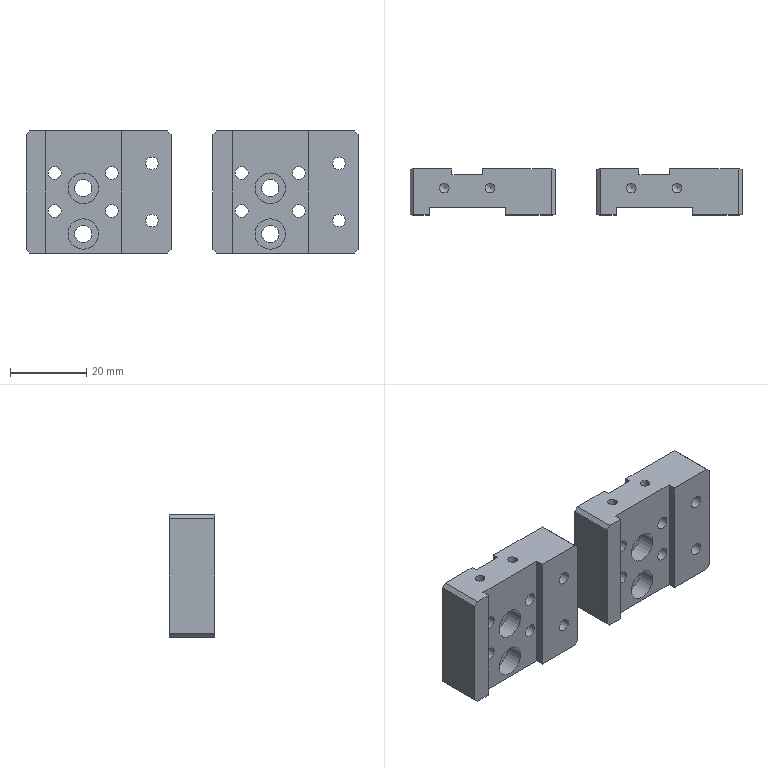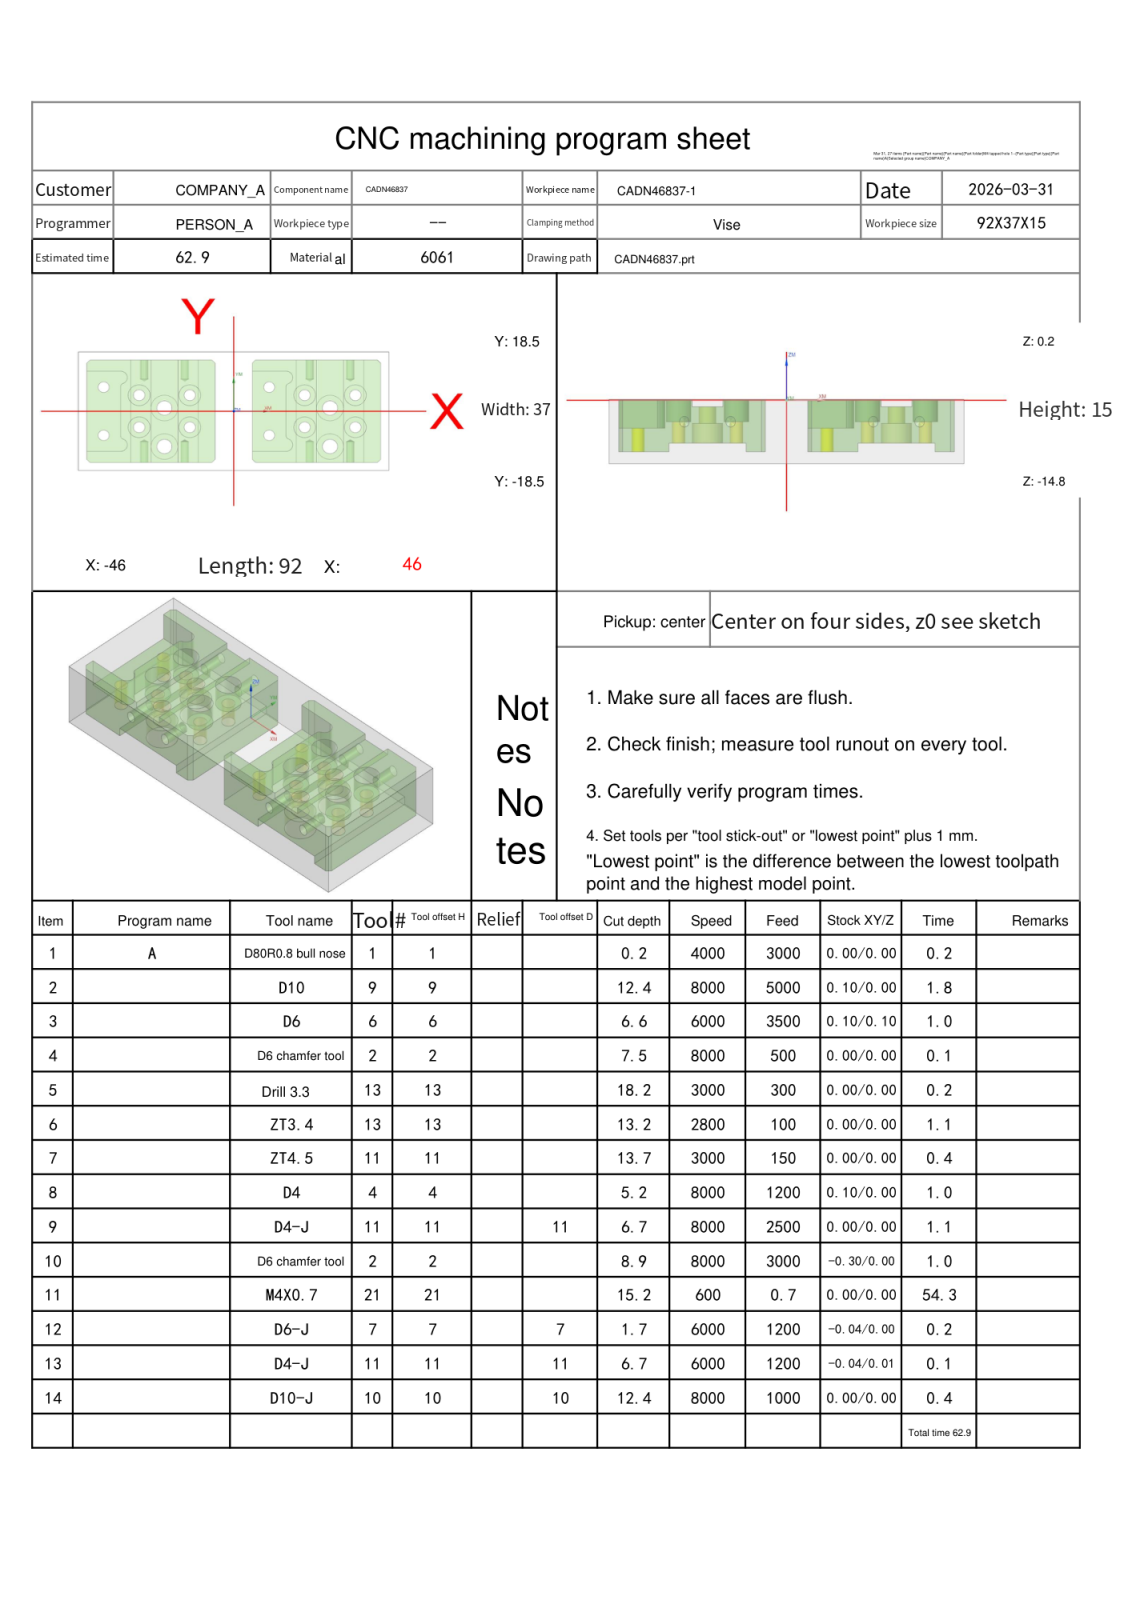NC program | NX | posted by the shop | part box 87 x 12 x 32 mm
Lines 2026 to 3069 of 5636:
N9 T11 M06
(D4-J  D=4. R=0. H=11 ce=0.00 di=0.00)
G00 G90 G54 X-28. Y5. M03 S8000
G43 H11 Z20.
M08
Z.5
G41 D11
G01 X-28.062 Y5.19 F500.
G03 X-28.641 Y5.609 I-.579 J-.19
X-29.25 Y5. I0.0 J-.609
X-29.25 Y5. Z-4.5 I1.25 J0.0
X-29.011 Y4.265 Z-5. I1.25 J0.0
X-28. Y3.75 I1.011 J.735
X-26.75 Y5. I0.0 J1.25
X-28. Y6.25 I-1.25 J0.0
X-29.25 Y5. I0.0 J-1.25
X-29.011 Y4.265 I1.25 J0.0
X-28.519 Y4.014 I.493 J.358
X-27.91 Y4.623 I0.0 J.609
G01 X-27.939 Y4.81
G40 X-28. Y5.
G00 Z20.
Y-5.
Z.5
G41 D11
G01 X-28.062 Y-4.81
G03 X-28.641 Y-4.391 I-.579 J-.19
X-29.25 Y-5. I0.0 J-.609
X-29.25 Y-5. Z-4.5 I1.25 J0.0
X-29.011 Y-5.735 Z-5. I1.25 J0.0
X-28. Y-6.25 I1.011 J.735
X-26.75 Y-5. I0.0 J1.25
X-28. Y-3.75 I-1.25 J0.0
X-29.25 Y-5. I0.0 J-1.25
X-29.011 Y-5.735 I1.25 J0.0
X-28.519 Y-5.986 I.493 J.358
X-27.91 Y-5.377 I0.0 J.609
G01 X-27.939 Y-5.19
G40 X-28. Y-5.
G00 Z20.
X-13.
Z.5
G41 D11
G01 X-13.062 Y-4.81
G03 X-13.641 Y-4.391 I-.579 J-.19
X-14.25 Y-5. I0.0 J-.609
X-14.25 Y-5. Z-4.5 I1.25 J0.0
X-14.011 Y-5.735 Z-5. I1.25 J0.0
X-13. Y-6.25 I1.011 J.735
X-11.75 Y-5. I0.0 J1.25
X-13. Y-3.75 I-1.25 J0.0
X-14.25 Y-5. I0.0 J-1.25
X-14.011 Y-5.735 I1.25 J0.0
X-13.519 Y-5.986 I.493 J.358
X-12.91 Y-5.377 I0.0 J.609
G01 X-12.939 Y-5.19
G40 X-13. Y-5.
G00 Z20.
Y5.
Z.5
G41 D11
G01 X-13.062 Y5.19
G03 X-13.641 Y5.609 I-.579 J-.19
X-14.25 Y5. I0.0 J-.609
X-14.25 Y5. Z-4.5 I1.25 J0.0
X-14.011 Y4.265 Z-5. I1.25 J0.0
X-13. Y3.75 I1.011 J.735
X-11.75 Y5. I0.0 J1.25
X-13. Y6.25 I-1.25 J0.0
X-14.25 Y5. I0.0 J-1.25
X-14.011 Y4.265 I1.25 J0.0
X-13.519 Y4.014 I.493 J.358
X-12.91 Y4.623 I0.0 J.609
G01 X-12.939 Y4.81
G40 X-13. Y5.
G00 Z20.
X21.
Z.5
G41 D11
G01 X20.938 Y5.19
G03 X20.359 Y5.609 I-.579 J-.19
X19.75 Y5. I0.0 J-.609
X19.75 Y5. Z-4.5 I1.25 J0.0
X19.989 Y4.265 Z-5. I1.25 J0.0
X21. Y3.75 I1.011 J.735
X22.25 Y5. I0.0 J1.25
X21. Y6.25 I-1.25 J0.0
X19.75 Y5. I0.0 J-1.25
X19.989 Y4.265 I1.25 J0.0
X20.481 Y4.014 I.493 J.358
X21.09 Y4.623 I0.0 J.609
G01 X21.061 Y4.81
G40 X21. Y5.
G00 Z20.
Y-5.
Z.5
G41 D11
G01 X20.938 Y-4.81
G03 X20.359 Y-4.391 I-.579 J-.19
X19.75 Y-5. I0.0 J-.609
X19.75 Y-5. Z-4.5 I1.25 J0.0
X19.989 Y-5.735 Z-5. I1.25 J0.0
X21. Y-6.25 I1.011 J.735
X22.25 Y-5. I0.0 J1.25
X21. Y-3.75 I-1.25 J0.0
X19.75 Y-5. I0.0 J-1.25
X19.989 Y-5.735 I1.25 J0.0
X20.481 Y-5.986 I.493 J.358
X21.09 Y-5.377 I0.0 J.609
G01 X21.061 Y-5.19
G40 X21. Y-5.
G00 Z20.
X36.
Z.5
G41 D11
G01 X35.938 Y-4.81
G03 X35.359 Y-4.391 I-.579 J-.19
X34.75 Y-5. I0.0 J-.609
X34.75 Y-5. Z-4.5 I1.25 J0.0
X34.989 Y-5.735 Z-5. I1.25 J0.0
X36. Y-6.25 I1.011 J.735
X37.25 Y-5. I0.0 J1.25
X36. Y-3.75 I-1.25 J0.0
X34.75 Y-5. I0.0 J-1.25
X34.989 Y-5.735 I1.25 J0.0
X35.481 Y-5.986 I.493 J.358
X36.09 Y-5.377 I0.0 J.609
G01 X36.061 Y-5.19
G40 X36. Y-5.
G00 Z20.
Y5.
Z.5
G41 D11
G01 X35.938 Y5.19
G03 X35.359 Y5.609 I-.579 J-.19
X34.75 Y5. I0.0 J-.609
X34.75 Y5. Z-4.5 I1.25 J0.0
X34.989 Y4.265 Z-5. I1.25 J0.0
X36. Y3.75 I1.011 J.735
X37.25 Y5. I0.0 J1.25
X36. Y6.25 I-1.25 J0.0
X34.75 Y5. I0.0 J-1.25
X34.989 Y4.265 I1.25 J0.0
X35.481 Y4.014 I.493 J.358
X36.09 Y4.623 I0.0 J.609
G01 X36.061 Y4.81
G40 X36. Y5.
G00 Z20.
G00 G90 X-39.064 Y-9.895 M03 S6000
Z20.
Z.305
G01 X-39.063 Y-9.902 Z.219 F2000.
X-39.059 Y-9.921 Z.141
X-39.053 Y-9.951 Z.071
X-39.045 Y-9.989 Z.009
X-39.033 Y-10.035 Z-.047
X-39.018 Y-10.086 Z-.096
X-39. Y-10.141 Z-.139
X-38.978 Y-10.197 Z-.175
X-38.953 Y-10.254 Z-.206
X-38.924 Y-10.309 Z-.232
X-38.89 Y-10.36 Z-.253
X-38.852 Y-10.405 Z-.269
X-38.81 Y-10.444 Z-.281
X-38.763 Y-10.474 Z-.289
X-38.71 Y-10.493 Z-.294
X-38.653 Y-10.5 Z-.295
X-33.5 F2500.
G02 X-35.5 Y-7.672 I1. J2.828
G01 Y-7.316
X-35.516 Y-7.273 Z-.296
X-35.562 Y-7.252 Z-.299
X-35.634 Y-7.251 Z-.303
X-35.73 Y-7.27 Z-.308
X-35.844 Y-7.305 Z-.315
X-35.975 Y-7.356 Z-.323
X-36.119 Y-7.42 Z-.332
X-36.272 Y-7.496 Z-.342
X-36.514 Y-7.632 Z-.358
X-36.753 Y-7.781 Z-.375
X-37.091 Y-8.025 Z-.402
X-37.407 Y-8.295 Z-.429
X-37.7 Y-8.588 Z-.457
X-37.967 Y-8.905 Z-.484
X-38.208 Y-9.244 Z-.51
X-38.309 Y-9.405 Z-.522
X-38.402 Y-9.566 Z-.533
X-38.486 Y-9.726 Z-.544
X-38.56 Y-9.879 Z-.554
X-38.622 Y-10.023 Z-.563
X-38.67 Y-10.155 Z-.57
X-38.704 Y-10.27 Z-.577
X-38.72 Y-10.365 Z-.583
X-38.718 Y-10.438 Z-.587
X-38.696 Y-10.484 Z-.59
X-38.653 Y-10.5
X-33.5
G02 X-35.5 Y-7.672 I1. J2.828
G01 Y-7.316
X-35.516 Y-7.273 Z-.591
X-35.562 Y-7.252 Z-.594
X-35.634 Y-7.251 Z-.598
X-35.73 Y-7.27 Z-.604
X-35.844 Y-7.305 Z-.61
X-35.975 Y-7.356 Z-.618
X-36.119 Y-7.42 Z-.627
X-36.272 Y-7.496 Z-.637
X-36.514 Y-7.632 Z-.653
X-36.753 Y-7.781 Z-.67
X-37.091 Y-8.025 Z-.697
X-37.407 Y-8.295 Z-.724
X-37.7 Y-8.588 Z-.752
X-37.967 Y-8.905 Z-.779
X-38.208 Y-9.244 Z-.806
X-38.309 Y-9.405 Z-.817
X-38.402 Y-9.566 Z-.828
X-38.486 Y-9.726 Z-.839
X-38.56 Y-9.879 Z-.849
X-38.622 Y-10.023 Z-.858
X-38.67 Y-10.155 Z-.866
X-38.704 Y-10.27 Z-.873
X-38.72 Y-10.365 Z-.878
X-38.718 Y-10.438 Z-.882
X-38.696 Y-10.484 Z-.885
X-38.653 Y-10.5 Z-.886
X-33.5
G02 X-35.5 Y-7.672 I1. J2.828
G01 Y-7.316
X-35.516 Y-7.273 Z-.887
X-35.562 Y-7.252 Z-.889
X-35.634 Y-7.251 Z-.893
X-35.73 Y-7.27 Z-.899
X-35.844 Y-7.305 Z-.906
X-35.975 Y-7.356 Z-.914
X-36.119 Y-7.42 Z-.923
X-36.272 Y-7.496 Z-.932
X-36.514 Y-7.632 Z-.949
X-36.753 Y-7.781 Z-.966
X-37.091 Y-8.025 Z-.992
X-37.407 Y-8.295 Z-1.019
X-37.7 Y-8.588 Z-1.047
X-37.967 Y-8.905 Z-1.074
X-38.208 Y-9.244 Z-1.101
X-38.309 Y-9.405 Z-1.113
X-38.402 Y-9.566 Z-1.124
X-38.486 Y-9.726 Z-1.134
X-38.56 Y-9.879 Z-1.144
X-38.622 Y-10.023 Z-1.153
X-38.67 Y-10.155 Z-1.161
X-38.704 Y-10.27 Z-1.168
X-38.72 Y-10.365 Z-1.173
X-38.718 Y-10.438 Z-1.177
X-38.696 Y-10.484 Z-1.18
X-38.653 Y-10.5 Z-1.181
X-33.5
G02 X-35.5 Y-7.672 I1. J2.828
G01 Y-7.316
X-35.516 Y-7.273 Z-1.182
X-35.562 Y-7.252 Z-1.184
X-35.634 Y-7.251 Z-1.189
X-35.73 Y-7.27 Z-1.194
X-35.844 Y-7.305 Z-1.201
X-35.975 Y-7.356 Z-1.209
X-36.119 Y-7.42 Z-1.218
X-36.272 Y-7.496 Z-1.228
X-36.514 Y-7.632 Z-1.244
X-36.753 Y-7.781 Z-1.261
X-37.091 Y-8.025 Z-1.287
X-37.407 Y-8.295 Z-1.315
X-37.7 Y-8.588 Z-1.342
X-37.967 Y-8.905 Z-1.37
X-38.208 Y-9.244 Z-1.396
X-38.309 Y-9.405 Z-1.408
X-38.402 Y-9.566 Z-1.419
X-38.486 Y-9.726 Z-1.429
X-38.56 Y-9.879 Z-1.439
X-38.622 Y-10.023 Z-1.448
X-38.67 Y-10.155 Z-1.456
X-38.704 Y-10.27 Z-1.463
X-38.72 Y-10.365 Z-1.469
X-38.718 Y-10.438 Z-1.473
X-38.696 Y-10.484 Z-1.475
X-38.653 Y-10.5 Z-1.476
X-33.5
G02 X-35.5 Y-7.672 I1. J2.828
G01 Y-7.316
X-35.516 Y-7.273 Z-1.477
X-35.562 Y-7.252 Z-1.48
X-35.634 Y-7.251 Z-1.484
X-35.73 Y-7.27 Z-1.489
X-35.844 Y-7.305 Z-1.496
X-35.975 Y-7.356 Z-1.504
X-36.119 Y-7.42 Z-1.513
X-36.272 Y-7.496 Z-1.523
X-36.514 Y-7.632 Z-1.539
X-36.753 Y-7.781 Z-1.556
X-37.091 Y-8.025 Z-1.583
X-37.407 Y-8.295 Z-1.61
X-37.7 Y-8.588 Z-1.638
X-37.967 Y-8.905 Z-1.665
X-38.208 Y-9.244 Z-1.691
X-38.309 Y-9.405 Z-1.703
X-38.402 Y-9.566 Z-1.714
X-38.486 Y-9.726 Z-1.725
X-38.56 Y-9.879 Z-1.734
X-38.622 Y-10.023 Z-1.743
X-38.67 Y-10.155 Z-1.751
X-38.704 Y-10.27 Z-1.758
X-38.72 Y-10.365 Z-1.764
X-38.718 Y-10.438 Z-1.768
X-38.696 Y-10.484 Z-1.77
X-38.653 Y-10.5 Z-1.771
X-33.5
G02 X-35.5 Y-7.672 I1. J2.828
G01 Y-7.316
X-35.516 Y-7.273 Z-1.772
X-35.562 Y-7.252 Z-1.775
X-35.634 Y-7.251 Z-1.779
X-35.73 Y-7.27 Z-1.785
X-35.844 Y-7.305 Z-1.791
X-35.975 Y-7.356 Z-1.799
X-36.119 Y-7.42 Z-1.808
X-36.272 Y-7.496 Z-1.818
X-36.514 Y-7.632 Z-1.834
X-36.753 Y-7.781 Z-1.851
X-37.091 Y-8.025 Z-1.878
X-37.407 Y-8.295 Z-1.905
X-37.7 Y-8.588 Z-1.933
X-37.967 Y-8.905 Z-1.96
X-38.208 Y-9.244 Z-1.987
X-38.309 Y-9.405 Z-1.998
X-38.402 Y-9.566 Z-2.009
X-38.486 Y-9.726 Z-2.02
X-38.56 Y-9.879 Z-2.03
X-38.622 Y-10.023 Z-2.039
X-38.67 Y-10.155 Z-2.047
X-38.704 Y-10.27 Z-2.053
X-38.72 Y-10.365 Z-2.059
X-38.718 Y-10.438 Z-2.063
X-38.696 Y-10.484 Z-2.066
X-38.653 Y-10.5 Z-2.067
X-33.5
G02 X-35.5 Y-7.672 I1. J2.828
G01 Y-7.316
X-35.516 Y-7.273
X-35.562 Y-7.252 Z-2.07
X-35.634 Y-7.251 Z-2.074
X-35.73 Y-7.27 Z-2.08
X-35.844 Y-7.305 Z-2.087
X-35.975 Y-7.356 Z-2.095
X-36.119 Y-7.42 Z-2.103
X-36.272 Y-7.496 Z-2.113
X-36.514 Y-7.632 Z-2.13
X-36.753 Y-7.781 Z-2.147
X-37.091 Y-8.025 Z-2.173
X-37.407 Y-8.295 Z-2.2
X-37.7 Y-8.588 Z-2.228
X-37.967 Y-8.905 Z-2.255
X-38.208 Y-9.244 Z-2.282
X-38.309 Y-9.405 Z-2.293
X-38.402 Y-9.566 Z-2.305
X-38.486 Y-9.726 Z-2.315
X-38.56 Y-9.879 Z-2.325
X-38.622 Y-10.023 Z-2.334
X-38.67 Y-10.155 Z-2.342
X-38.704 Y-10.27 Z-2.349
X-38.72 Y-10.365 Z-2.354
X-38.718 Y-10.438 Z-2.358
X-38.696 Y-10.484 Z-2.361
X-38.653 Y-10.5 Z-2.362
X-33.5
G02 X-35.5 Y-7.672 I1. J2.828
G01 Y-7.316
X-35.516 Y-7.273 Z-2.363
X-35.562 Y-7.252 Z-2.365
X-35.634 Y-7.251 Z-2.369
X-35.73 Y-7.27 Z-2.375
X-35.844 Y-7.305 Z-2.382
X-35.975 Y-7.356 Z-2.39
X-36.119 Y-7.42 Z-2.399
X-36.272 Y-7.496 Z-2.409
X-36.514 Y-7.632 Z-2.425
X-36.753 Y-7.781 Z-2.442
X-37.091 Y-8.025 Z-2.468
X-37.407 Y-8.295 Z-2.496
X-37.7 Y-8.588 Z-2.523
X-37.967 Y-8.905 Z-2.551
X-38.208 Y-9.244 Z-2.577
X-38.309 Y-9.405 Z-2.589
X-38.402 Y-9.566 Z-2.6
X-38.486 Y-9.726 Z-2.61
X-38.56 Y-9.879 Z-2.62
X-38.622 Y-10.023 Z-2.629
X-38.67 Y-10.155 Z-2.637
X-38.704 Y-10.27 Z-2.644
X-38.72 Y-10.365 Z-2.649
X-38.718 Y-10.438 Z-2.654
X-38.696 Y-10.484 Z-2.656
X-38.653 Y-10.5 Z-2.657
X-33.5
G02 X-35.5 Y-7.672 I1. J2.828
G01 Y-7.316
X-35.516 Y-7.273 Z-2.658
X-35.562 Y-7.252 Z-2.661
X-35.634 Y-7.251 Z-2.665
X-35.73 Y-7.27 Z-2.67
X-35.844 Y-7.305 Z-2.677
X-35.975 Y-7.356 Z-2.685
X-36.119 Y-7.42 Z-2.694
X-36.272 Y-7.496 Z-2.704
X-36.514 Y-7.632 Z-2.72
X-36.753 Y-7.781 Z-2.737
X-37.091 Y-8.025 Z-2.763
X-37.407 Y-8.295 Z-2.791
X-37.7 Y-8.588 Z-2.818
X-37.967 Y-8.905 Z-2.846
X-38.208 Y-9.244 Z-2.872
X-38.309 Y-9.405 Z-2.884
X-38.402 Y-9.566 Z-2.895
X-38.486 Y-9.726 Z-2.906
X-38.56 Y-9.879 Z-2.915
X-38.622 Y-10.023 Z-2.924
X-38.67 Y-10.155 Z-2.932
X-38.704 Y-10.27 Z-2.939
X-38.72 Y-10.365 Z-2.945
X-38.718 Y-10.438 Z-2.949
X-38.696 Y-10.484 Z-2.951
X-38.653 Y-10.5 Z-2.952
X-33.5
G02 X-35.5 Y-7.672 I1. J2.828
G01 Y-7.316
X-35.516 Y-7.273 Z-2.953
X-35.562 Y-7.252 Z-2.956
X-35.634 Y-7.251 Z-2.96
X-35.73 Y-7.27 Z-2.965
X-35.844 Y-7.305 Z-2.972
X-35.975 Y-7.356 Z-2.98
X-36.119 Y-7.42 Z-2.989
X-36.272 Y-7.496 Z-2.999
X-36.514 Y-7.632 Z-3.015
X-36.753 Y-7.781 Z-3.032
X-37.091 Y-8.025 Z-3.059
X-37.407 Y-8.295 Z-3.086
X-37.7 Y-8.588 Z-3.114
X-37.967 Y-8.905 Z-3.141
X-38.208 Y-9.244 Z-3.168
X-38.309 Y-9.405 Z-3.179
X-38.402 Y-9.566 Z-3.19
X-38.486 Y-9.726 Z-3.201
X-38.56 Y-9.879 Z-3.211
X-38.622 Y-10.023 Z-3.22
X-38.67 Y-10.155 Z-3.228
X-38.704 Y-10.27 Z-3.234
X-38.72 Y-10.365 Z-3.24
X-38.718 Y-10.438 Z-3.244
X-38.696 Y-10.484 Z-3.247
X-38.653 Y-10.5 Z-3.248
X-33.5
G02 X-35.5 Y-7.672 I1. J2.828
G01 Y-7.316
X-35.516 Y-7.273
X-35.562 Y-7.252 Z-3.251
X-35.634 Y-7.251 Z-3.255
X-35.73 Y-7.27 Z-3.261
X-35.844 Y-7.305 Z-3.267
X-35.975 Y-7.356 Z-3.275
X-36.119 Y-7.42 Z-3.284
X-36.272 Y-7.496 Z-3.294
X-36.514 Y-7.632 Z-3.31
X-36.753 Y-7.781 Z-3.327
X-37.091 Y-8.025 Z-3.354
X-37.407 Y-8.295 Z-3.381
X-37.7 Y-8.588 Z-3.409
X-37.967 Y-8.905 Z-3.436
X-38.208 Y-9.244 Z-3.463
X-38.309 Y-9.405 Z-3.474
X-38.402 Y-9.566 Z-3.485
X-38.486 Y-9.726 Z-3.496
X-38.56 Y-9.879 Z-3.506
X-38.622 Y-10.023 Z-3.515
X-38.67 Y-10.155 Z-3.523
X-38.704 Y-10.27 Z-3.53
X-38.72 Y-10.365 Z-3.535
X-38.718 Y-10.438 Z-3.539
X-38.696 Y-10.484 Z-3.542
X-38.653 Y-10.5 Z-3.543
X-33.5
G02 X-35.5 Y-7.672 I1. J2.828
G01 Y-7.316
X-35.516 Y-7.273 Z-3.544
X-35.562 Y-7.252 Z-3.546
X-35.634 Y-7.251 Z-3.55
X-35.73 Y-7.27 Z-3.556
X-35.844 Y-7.305 Z-3.563
X-35.975 Y-7.356 Z-3.571
X-36.119 Y-7.42 Z-3.58
X-36.272 Y-7.496 Z-3.589
X-36.514 Y-7.632 Z-3.606
X-36.753 Y-7.781 Z-3.623
X-37.091 Y-8.025 Z-3.649
X-37.407 Y-8.295 Z-3.677
X-37.7 Y-8.588 Z-3.704
X-37.967 Y-8.905 Z-3.732
X-38.208 Y-9.244 Z-3.758
X-38.309 Y-9.405 Z-3.77
X-38.402 Y-9.566 Z-3.781
X-38.486 Y-9.726 Z-3.791
X-38.56 Y-9.879 Z-3.801
X-38.622 Y-10.023 Z-3.81
X-38.67 Y-10.155 Z-3.818
X-38.704 Y-10.27 Z-3.825
X-38.72 Y-10.365 Z-3.83
X-38.718 Y-10.438 Z-3.834
X-38.696 Y-10.484 Z-3.837
X-38.653 Y-10.5 Z-3.838
X-33.5
G02 X-35.5 Y-7.672 I1. J2.828
G01 Y-7.316
X-35.516 Y-7.273 Z-3.839
X-35.562 Y-7.252 Z-3.841
X-35.634 Y-7.251 Z-3.846
X-35.73 Y-7.27 Z-3.851
X-35.844 Y-7.305 Z-3.858
X-35.975 Y-7.356 Z-3.866
X-36.119 Y-7.42 Z-3.875
X-36.272 Y-7.496 Z-3.885
X-36.514 Y-7.632 Z-3.901
X-36.753 Y-7.781 Z-3.918
X-37.091 Y-8.025 Z-3.944
X-37.407 Y-8.295 Z-3.972
X-37.7 Y-8.588 Z-3.999
X-37.967 Y-8.905 Z-4.027
X-38.208 Y-9.244 Z-4.053
X-38.309 Y-9.405 Z-4.065
X-38.402 Y-9.566 Z-4.076
X-38.486 Y-9.726 Z-4.086
X-38.56 Y-9.879 Z-4.096
X-38.622 Y-10.023 Z-4.105
X-38.67 Y-10.155 Z-4.113
X-38.704 Y-10.27 Z-4.12
X-38.72 Y-10.365 Z-4.126
X-38.718 Y-10.438 Z-4.13
X-38.696 Y-10.484 Z-4.132
X-38.653 Y-10.5 Z-4.133
X-33.5
G02 X-35.5 Y-7.672 I1. J2.828
G01 Y-7.316
X-35.516 Y-7.273 Z-4.134
X-35.562 Y-7.252 Z-4.137
X-35.634 Y-7.251 Z-4.141
X-35.73 Y-7.27 Z-4.146
X-35.844 Y-7.305 Z-4.153
X-35.975 Y-7.356 Z-4.161
X-36.119 Y-7.42 Z-4.17
X-36.272 Y-7.496 Z-4.18
X-36.514 Y-7.632 Z-4.196
X-36.753 Y-7.781 Z-4.213
X-37.091 Y-8.025 Z-4.24
X-37.407 Y-8.295 Z-4.267
X-37.7 Y-8.588 Z-4.295
X-37.967 Y-8.905 Z-4.322
X-38.208 Y-9.244 Z-4.348
X-38.309 Y-9.405 Z-4.36
X-38.402 Y-9.566 Z-4.371
X-38.486 Y-9.726 Z-4.382
X-38.56 Y-9.879 Z-4.392
X-38.622 Y-10.023 Z-4.4
X-38.67 Y-10.155 Z-4.408
X-38.704 Y-10.27 Z-4.415
X-38.72 Y-10.365 Z-4.421
X-38.718 Y-10.438 Z-4.425
X-38.696 Y-10.484 Z-4.428
X-38.653 Y-10.5
X-33.5
G02 X-35.5 Y-7.672 I1. J2.828
G01 Y-7.316
X-35.516 Y-7.273 Z-4.429
X-35.562 Y-7.252 Z-4.432
X-35.634 Y-7.251 Z-4.436
X-35.73 Y-7.27 Z-4.442
X-35.844 Y-7.305 Z-4.448
X-35.975 Y-7.356 Z-4.456
X-36.119 Y-7.42 Z-4.465
X-36.272 Y-7.496 Z-4.475
X-36.514 Y-7.632 Z-4.491
X-36.753 Y-7.781 Z-4.508
X-37.091 Y-8.025 Z-4.535
X-37.407 Y-8.295 Z-4.562
X-37.7 Y-8.588 Z-4.59
X-37.967 Y-8.905 Z-4.617
X-38.208 Y-9.244 Z-4.644
X-38.309 Y-9.405 Z-4.655
X-38.402 Y-9.566 Z-4.666
X-38.486 Y-9.726 Z-4.677
X-38.56 Y-9.879 Z-4.687
X-38.622 Y-10.023 Z-4.696
X-38.67 Y-10.155 Z-4.704
X-38.704 Y-10.27 Z-4.71
X-38.72 Y-10.365 Z-4.716
X-38.718 Y-10.438 Z-4.72
X-38.696 Y-10.484 Z-4.723
X-38.653 Y-10.5 Z-4.724
X-33.5
G02 X-35.5 Y-7.672 I1. J2.828
G01 Y-7.316
X-35.516 Y-7.273 Z-4.725
X-35.562 Y-7.252 Z-4.727
X-35.634 Y-7.251 Z-4.731
X-35.73 Y-7.27 Z-4.737
X-35.844 Y-7.305 Z-4.744
X-35.975 Y-7.356 Z-4.752
X-36.119 Y-7.42 Z-4.761
X-36.272 Y-7.496 Z-4.77
X-36.514 Y-7.632 Z-4.787
X-36.753 Y-7.781 Z-4.804
X-37.091 Y-8.025 Z-4.83
X-37.407 Y-8.295 Z-4.857
X-37.7 Y-8.588 Z-4.885
X-37.967 Y-8.905 Z-4.912
X-38.208 Y-9.244 Z-4.939
X-38.309 Y-9.405 Z-4.95
X-38.402 Y-9.566 Z-4.962
X-38.486 Y-9.726 Z-4.972
X-38.56 Y-9.879 Z-4.982
X-38.622 Y-10.023 Z-4.991
X-38.67 Y-10.155 Z-4.999
X-38.704 Y-10.27 Z-5.006
X-38.72 Y-10.365 Z-5.011
X-38.718 Y-10.438 Z-5.015
X-38.696 Y-10.484 Z-5.018
X-38.653 Y-10.5 Z-5.019
X-33.5
G02 X-35.5 Y-7.672 I1. J2.828
G01 Y-7.316
X-35.516 Y-7.273 Z-5.02
X-35.562 Y-7.252 Z-5.022
X-35.634 Y-7.251 Z-5.026
X-35.73 Y-7.27 Z-5.032
X-35.844 Y-7.305 Z-5.039
X-35.975 Y-7.356 Z-5.047
X-36.119 Y-7.42 Z-5.056
X-36.272 Y-7.496 Z-5.066
X-36.514 Y-7.632 Z-5.082
X-36.753 Y-7.781 Z-5.099
X-37.091 Y-8.025 Z-5.125
X-37.407 Y-8.295 Z-5.153
X-37.7 Y-8.588 Z-5.18
X-37.967 Y-8.905 Z-5.208
X-38.208 Y-9.244 Z-5.234
X-38.309 Y-9.405 Z-5.246
X-38.402 Y-9.566 Z-5.257
X-38.486 Y-9.726 Z-5.267
X-38.56 Y-9.879 Z-5.277
X-38.622 Y-10.023 Z-5.286
X-38.67 Y-10.155 Z-5.294
X-38.704 Y-10.27 Z-5.301
X-38.72 Y-10.365 Z-5.306
X-38.718 Y-10.438 Z-5.311
X-38.696 Y-10.484 Z-5.313
X-38.653 Y-10.5 Z-5.314
X-33.5
G02 X-35.5 Y-7.672 I1. J2.828
G01 Y-7.316
X-35.516 Y-7.273 Z-5.315
X-35.562 Y-7.252 Z-5.318
X-35.634 Y-7.251 Z-5.322
X-35.73 Y-7.27 Z-5.327
X-35.844 Y-7.305 Z-5.334
X-35.975 Y-7.356 Z-5.342
X-36.119 Y-7.42 Z-5.351
X-36.272 Y-7.496 Z-5.361
X-36.514 Y-7.632 Z-5.377
X-36.753 Y-7.781 Z-5.394
X-37.091 Y-8.025 Z-5.421
X-37.407 Y-8.295 Z-5.448
X-37.7 Y-8.588 Z-5.476
X-37.967 Y-8.905 Z-5.503
X-38.208 Y-9.244 Z-5.529
X-38.309 Y-9.405 Z-5.541
X-38.402 Y-9.566 Z-5.552
X-38.486 Y-9.726 Z-5.563
X-38.56 Y-9.879 Z-5.572
X-38.622 Y-10.023 Z-5.581
X-38.67 Y-10.155 Z-5.589
X-38.704 Y-10.27 Z-5.596
X-38.72 Y-10.365 Z-5.602
X-38.718 Y-10.438 Z-5.606
X-38.696 Y-10.484 Z-5.608
X-38.653 Y-10.5 Z-5.609
X-33.5
G02 X-35.5 Y-7.672 I1. J2.828
G01 Y-7.316
X-35.516 Y-7.273 Z-5.61
X-35.562 Y-7.252 Z-5.613
X-35.634 Y-7.251 Z-5.617
X-35.73 Y-7.27 Z-5.622
X-35.844 Y-7.305 Z-5.629
X-35.975 Y-7.356 Z-5.637
X-36.119 Y-7.42 Z-5.646
X-36.272 Y-7.496 Z-5.656
X-36.514 Y-7.632 Z-5.672
X-36.753 Y-7.781 Z-5.689
X-37.091 Y-8.025 Z-5.716
X-37.407 Y-8.295 Z-5.743
X-37.7 Y-8.588 Z-5.771
X-37.967 Y-8.905 Z-5.798
X-38.208 Y-9.244 Z-5.825
X-38.309 Y-9.405 Z-5.836
X-38.402 Y-9.566 Z-5.847
X-38.486 Y-9.726 Z-5.858
X-38.56 Y-9.879 Z-5.868
X-38.622 Y-10.023 Z-5.877
X-38.67 Y-10.155 Z-5.885
X-38.704 Y-10.27 Z-5.891
X-38.72 Y-10.365 Z-5.897
X-38.718 Y-10.438 Z-5.901
X-38.696 Y-10.484 Z-5.904
X-38.653 Y-10.5 Z-5.905
X-33.5
G02 X-35.5 Y-7.672 I1. J2.828
G01 Y-7.316
X-35.516 Y-7.273
X-35.562 Y-7.252 Z-5.908
X-35.634 Y-7.251 Z-5.912
X-35.73 Y-7.27 Z-5.918
X-35.844 Y-7.305 Z-5.925
X-35.975 Y-7.356 Z-5.932
X-36.119 Y-7.42 Z-5.941
X-36.272 Y-7.496 Z-5.951
X-36.514 Y-7.632 Z-5.968
X-36.753 Y-7.781 Z-5.985
X-37.091 Y-8.025 Z-6.011
X-37.407 Y-8.295 Z-6.038
X-37.7 Y-8.588 Z-6.066
X-37.967 Y-8.905 Z-6.093
X-38.208 Y-9.244 Z-6.12
X-38.309 Y-9.405 Z-6.131
X-38.402 Y-9.566 Z-6.143
X-38.486 Y-9.726 Z-6.153
X-38.56 Y-9.879 Z-6.163
X-38.622 Y-10.023 Z-6.172
X-38.67 Y-10.155 Z-6.18
X-38.704 Y-10.27 Z-6.187
X-38.72 Y-10.365 Z-6.192
X-38.718 Y-10.438 Z-6.196
X-38.696 Y-10.484 Z-6.199
X-38.653 Y-10.5 Z-6.2
X-33.5
G02 X-35.5 Y-7.672 I1. J2.828
G01 Y-7.316
X-35.516 Y-7.273 Z-6.201
X-35.562 Y-7.252 Z-6.203
X-35.634 Y-7.251 Z-6.207
X-35.73 Y-7.27 Z-6.213
X-35.844 Y-7.305 Z-6.22
X-35.975 Y-7.356 Z-6.228
X-36.119 Y-7.42 Z-6.237
X-36.272 Y-7.496 Z-6.247
X-36.514 Y-7.632 Z-6.263
X-36.753 Y-7.781 Z-6.28
X-37.091 Y-8.025 Z-6.306
X-37.407 Y-8.295 Z-6.334
X-37.7 Y-8.588 Z-6.361
X-37.967 Y-8.905 Z-6.389
X-38.208 Y-9.244 Z-6.415
X-38.309 Y-9.405 Z-6.427
X-38.402 Y-9.566 Z-6.438
X-38.486 Y-9.726 Z-6.448
X-38.56 Y-9.879 Z-6.458
X-38.622 Y-10.023 Z-6.467
X-38.67 Y-10.155 Z-6.475
X-38.704 Y-10.27 Z-6.482
X-38.72 Y-10.365 Z-6.487
X-38.718 Y-10.438 Z-6.492
X-38.696 Y-10.484 Z-6.494
X-38.653 Y-10.5 Z-6.495
X-33.5
G02 X-35.5 Y-7.672 I1. J2.828
G01 Y-7.316
X-35.507 Y-7.259 Z-6.494
X-35.526 Y-7.207 Z-6.489
X-35.555 Y-7.162 Z-6.481
X-35.594 Y-7.121 Z-6.469
X-35.639 Y-7.085 Z-6.453
X-35.69 Y-7.054 Z-6.432
X-35.744 Y-7.027 Z-6.406
X-35.8 Y-7.004 Z-6.375
X-35.856 Y-6.985 Z-6.338
X-35.91 Y-6.97 Z-6.296
X-35.961 Y-6.957 Z-6.247
X-36.006 Y-6.948 Z-6.191
X-36.045 Y-6.941 Z-6.129
X-36.074 Y-6.936 Z-6.059
X-36.093 Y-6.934 Z-5.981
X-36.1 Y-6.933 Z-5.895
G00 Z3.
Y6.916
Z.305
G01 X-36.094 Y6.917 Z.219 F2000.
X-36.075 Y6.92 Z.141
X-36.045 Y6.925 Z.071
X-36.007 Y6.933 Z.009
X-35.961 Y6.944 Z-.047
X-35.91 Y6.958 Z-.096
X-35.856 Y6.975 Z-.139
X-35.8 Y6.996 Z-.175
X-35.744 Y7.02 Z-.206
X-35.69 Y7.048 Z-.232
X-35.639 Y7.081 Z-.253
X-35.594 Y7.118 Z-.269
X-35.555 Y7.16 Z-.281
X-35.526 Y7.207 Z-.289
X-35.507 Y7.258 Z-.294
X-35.5 Y7.316 Z-.295
Y7.672 F2500.
G02 X-33.5 Y10.5 I3. J0.0
G01 X-38.653
X-38.696 Y10.484 Z-.296
X-38.718 Y10.438 Z-.299
X-38.719 Y10.365 Z-.303
X-38.702 Y10.27 Z-.308
X-38.669 Y10.154 Z-.315
X-38.62 Y10.023 Z-.323
X-38.557 Y9.878 Z-.332
X-38.483 Y9.725 Z-.342
X-38.398 Y9.565 Z-.352
X-38.304 Y9.403 Z-.364
X-38.203 Y9.242 Z-.375
X-37.962 Y8.901 Z-.402
X-37.695 Y8.583 Z-.429
X-37.403 Y8.288 Z-.457
X-37.088 Y8.018 Z-.484
X-36.75 Y7.774 Z-.51
X-36.59 Y7.672 Z-.522
X-36.429 Y7.577 Z-.533
X-36.27 Y7.491 Z-.544
X-36.118 Y7.416 Z-.554
X-35.974 Y7.352 Z-.563
X-35.844 Y7.302 Z-.57
X-35.729 Y7.268 Z-.577
X-35.634 Y7.25 Z-.583
X-35.562 Y7.251 Z-.587
X-35.516 Y7.273 Z-.59
X-35.5 Y7.316
Y7.672
G02 X-33.5 Y10.5 I3. J0.0
G01 X-38.653
X-38.696 Y10.484 Z-.591
X-38.718 Y10.438 Z-.594
X-38.719 Y10.365 Z-.598
X-38.702 Y10.27 Z-.604
X-38.669 Y10.154 Z-.61
X-38.62 Y10.023 Z-.618
X-38.557 Y9.878 Z-.627
X-38.483 Y9.725 Z-.637
X-38.398 Y9.565 Z-.648
X-38.304 Y9.403 Z-.659
X-38.203 Y9.242 Z-.67
X-37.962 Y8.901 Z-.697
X-37.695 Y8.583 Z-.724
X-37.403 Y8.288 Z-.752
X-37.088 Y8.018 Z-.779
X-36.75 Y7.774 Z-.806
X-36.59 Y7.672 Z-.817
X-36.429 Y7.577 Z-.828
X-36.27 Y7.491 Z-.839
X-36.118 Y7.416 Z-.849
X-35.974 Y7.352 Z-.858
X-35.844 Y7.302 Z-.866
X-35.729 Y7.268 Z-.873
X-35.634 Y7.25 Z-.878
X-35.562 Y7.251 Z-.882
X-35.516 Y7.273 Z-.885
X-35.5 Y7.316 Z-.886
Y7.672
G02 X-33.5 Y10.5 I3. J0.0
G01 X-38.653
X-38.696 Y10.484 Z-.887
X-38.718 Y10.438 Z-.889
X-38.719 Y10.365 Z-.893
X-38.702 Y10.27 Z-.899
X-38.669 Y10.154 Z-.906
X-38.62 Y10.023 Z-.914
X-38.557 Y9.878 Z-.923
X-38.483 Y9.725 Z-.932
X-38.398 Y9.565 Z-.943
X-38.304 Y9.403 Z-.954
X-38.203 Y9.242 Z-.966
X-37.962 Y8.901 Z-.992
X-37.695 Y8.583 Z-1.019
X-37.403 Y8.288 Z-1.047
X-37.088 Y8.018 Z-1.074
X-36.75 Y7.774 Z-1.101
X-36.59 Y7.672 Z-1.113
X-36.429 Y7.577 Z-1.124
X-36.27 Y7.491 Z-1.134
X-36.118 Y7.416 Z-1.144
X-35.974 Y7.352 Z-1.153
X-35.844 Y7.302 Z-1.161
X-35.729 Y7.268 Z-1.168
X-35.634 Y7.25 Z-1.173
X-35.562 Y7.251 Z-1.177
X-35.516 Y7.273 Z-1.18
X-35.5 Y7.316 Z-1.181
Y7.672
G02 X-33.5 Y10.5 I3. J0.0
G01 X-38.653
X-38.696 Y10.484 Z-1.182
X-38.718 Y10.438 Z-1.184
X-38.719 Y10.365 Z-1.189
X-38.702 Y10.27 Z-1.194
X-38.669 Y10.154 Z-1.201
X-38.62 Y10.023 Z-1.209
X-38.557 Y9.878 Z-1.218
X-38.483 Y9.725 Z-1.228
X-38.398 Y9.565 Z-1.238
X-38.304 Y9.403 Z-1.249
X-38.203 Y9.242 Z-1.261
X-37.962 Y8.901 Z-1.287
X-37.695 Y8.583 Z-1.315
X-37.403 Y8.288 Z-1.342
X-37.088 Y8.018 Z-1.37
X-36.75 Y7.774 Z-1.396
X-36.59 Y7.672 Z-1.408
X-36.429 Y7.577 Z-1.419
X-36.27 Y7.491 Z-1.429
X-36.118 Y7.416 Z-1.439
X-35.974 Y7.352 Z-1.448
X-35.844 Y7.302 Z-1.456
X-35.729 Y7.268 Z-1.463
X-35.634 Y7.25 Z-1.469
X-35.562 Y7.251 Z-1.473
X-35.516 Y7.273 Z-1.475
X-35.5 Y7.316 Z-1.476
Y7.672
G02 X-33.5 Y10.5 I3. J0.0
G01 X-38.653
X-38.696 Y10.484 Z-1.477
X-38.718 Y10.438 Z-1.48
X-38.719 Y10.365 Z-1.484
X-38.702 Y10.27 Z-1.489
X-38.669 Y10.154 Z-1.496
X-38.62 Y10.023 Z-1.504
X-38.557 Y9.878 Z-1.513
X-38.483 Y9.725 Z-1.523
X-38.398 Y9.565 Z-1.533
X-38.304 Y9.403 Z-1.545
X-38.203 Y9.242 Z-1.556
X-37.962 Y8.901 Z-1.583
X-37.695 Y8.583 Z-1.61
X-37.403 Y8.288 Z-1.638
X-37.088 Y8.018 Z-1.665
X-36.75 Y7.774 Z-1.691
X-36.59 Y7.672 Z-1.703
X-36.429 Y7.577 Z-1.714
X-36.27 Y7.491 Z-1.725
X-36.118 Y7.416 Z-1.734
X-35.974 Y7.352 Z-1.743
X-35.844 Y7.302 Z-1.751
X-35.729 Y7.268 Z-1.758
X-35.634 Y7.25 Z-1.764
X-35.562 Y7.251 Z-1.768
X-35.516 Y7.273 Z-1.77
X-35.5 Y7.316 Z-1.771
Y7.672
G02 X-33.5 Y10.5 I3. J0.0
G01 X-38.653
X-38.696 Y10.484 Z-1.772
X-38.718 Y10.438 Z-1.775
X-38.719 Y10.365 Z-1.779
X-38.702 Y10.27 Z-1.785
X-38.669 Y10.154 Z-1.791
X-38.62 Y10.023 Z-1.799
X-38.557 Y9.878 Z-1.808
X-38.483 Y9.725 Z-1.818
X-38.398 Y9.565 Z-1.829
X-38.304 Y9.403 Z-1.84
X-38.203 Y9.242 Z-1.851
X-37.962 Y8.901 Z-1.878
X-37.695 Y8.583 Z-1.905
X-37.403 Y8.288 Z-1.933
X-37.088 Y8.018 Z-1.96
X-36.75 Y7.774 Z-1.987
X-36.59 Y7.672 Z-1.998
X-36.429 Y7.577 Z-2.009
X-36.27 Y7.491 Z-2.02
X-36.118 Y7.416 Z-2.03
X-35.974 Y7.352 Z-2.039
X-35.844 Y7.302 Z-2.047
X-35.729 Y7.268 Z-2.053
X-35.634 Y7.25 Z-2.059
X-35.562 Y7.251 Z-2.063
X-35.516 Y7.273 Z-2.066
X-35.5 Y7.316 Z-2.067
Y7.672
G02 X-33.5 Y10.5 I3. J0.0
G01 X-38.653
X-38.696 Y10.484
X-38.718 Y10.438 Z-2.07
X-38.719 Y10.365 Z-2.074
X-38.702 Y10.27 Z-2.08
X-38.669 Y10.154 Z-2.087
X-38.62 Y10.023 Z-2.095
X-38.557 Y9.878 Z-2.103
X-38.483 Y9.725 Z-2.113
X-38.398 Y9.565 Z-2.124
X-38.304 Y9.403 Z-2.135
X-38.203 Y9.242 Z-2.147
X-37.962 Y8.901 Z-2.173
X-37.695 Y8.583 Z-2.2
X-37.403 Y8.288 Z-2.228
X-37.088 Y8.018 Z-2.255
X-36.75 Y7.774 Z-2.282
X-36.59 Y7.672 Z-2.293
X-36.429 Y7.577 Z-2.305
X-36.27 Y7.491 Z-2.315
X-36.118 Y7.416 Z-2.325
X-35.974 Y7.352 Z-2.334
X-35.844 Y7.302 Z-2.342
X-35.729 Y7.268 Z-2.349
X-35.634 Y7.25 Z-2.354
X-35.562 Y7.251 Z-2.358
X-35.516 Y7.273 Z-2.361
X-35.5 Y7.316 Z-2.362
Y7.672
G02 X-33.5 Y10.5 I3. J0.0
G01 X-38.653
X-38.696 Y10.484 Z-2.363
X-38.718 Y10.438 Z-2.365
X-38.719 Y10.365 Z-2.369
X-38.702 Y10.27 Z-2.375
X-38.669 Y10.154 Z-2.382
X-38.62 Y10.023 Z-2.39
X-38.557 Y9.878 Z-2.399
X-38.483 Y9.725 Z-2.409
X-38.398 Y9.565 Z-2.419
X-38.304 Y9.403 Z-2.43
X-38.203 Y9.242 Z-2.442
X-37.962 Y8.901 Z-2.468
X-37.695 Y8.583 Z-2.496
X-37.403 Y8.288 Z-2.523
X-37.088 Y8.018 Z-2.551
X-36.75 Y7.774 Z-2.577
X-36.59 Y7.672 Z-2.589